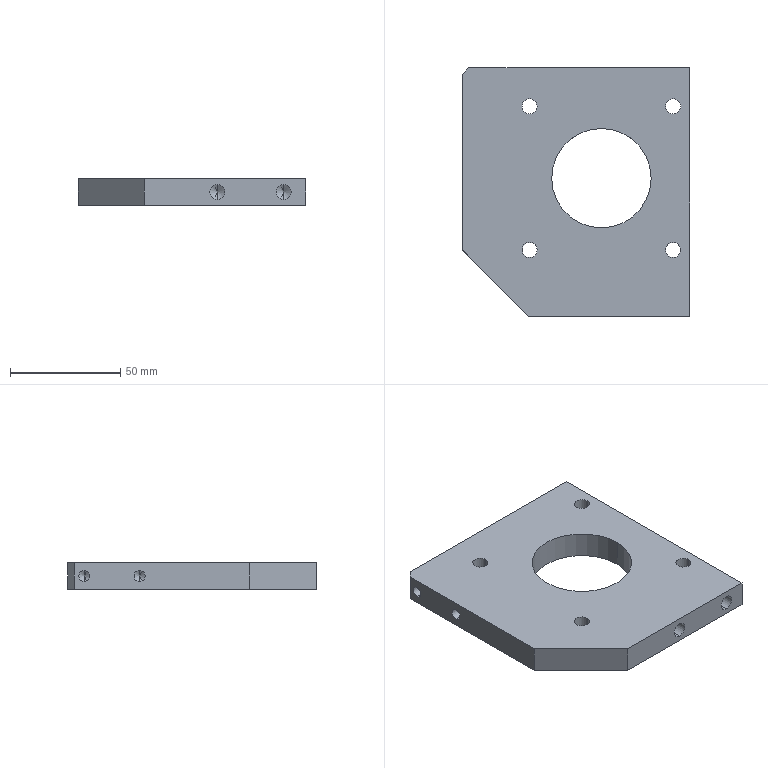Part | SolidWorks | features HoleWzd 3, Chamfer 2, ICE 2, 3DProfileFeature 1, Extrusion 1 | 1 solid | 34 faces | box 103 x 112.5 x 12 mm | volume 110488 mm3 | cylinder 18 | cone 8 | plane 8 | commonest cylinder face diameters 6.8 x12 5 x4 45 x2
STEP:
#1=CARTESIAN_POINT('',(-43.25,17.5,3.5));
#2=VERTEX_POINT('',#1);
#3=CARTESIAN_POINT('',(-43.25,17.5,8.5));
#4=VERTEX_POINT('',#3);
#5=CARTESIAN_POINT('',(-43.25,17.5,6.));
#6=DIRECTION('',(-1.,0.,0.));
#7=DIRECTION('',(0.,0.,1.));
#8=AXIS2_PLACEMENT_3D('',#5,#6,#7);
#9=CIRCLE('',#8,2.5);
#10=EDGE_CURVE('',#2,#4,#9,.T.);
#11=ORIENTED_EDGE('',*,*,#10,.F.);
#12=CARTESIAN_POINT('',(-63.,17.5,3.5));
#13=VERTEX_POINT('',#12);
#14=CARTESIAN_POINT('',(-63.,17.5,3.5));
#15=DIRECTION('',(-1.,0.,0.));
#16=VECTOR('',#15,1000.);
#17=LINE('',#14,#16);
#18=EDGE_CURVE('',#2,#13,#17,.T.);
#19=ORIENTED_EDGE('',*,*,#18,.T.);
#20=CARTESIAN_POINT('',(-63.,17.5,8.5));
#21=VERTEX_POINT('',#20);
#22=CARTESIAN_POINT('',(-63.,17.5,6.));
#23=DIRECTION('',(-1.,0.,0.));
#24=DIRECTION('',(0.,0.,1.));
#25=AXIS2_PLACEMENT_3D('',#22,#23,#24);
#26=CIRCLE('',#25,2.5);
#27=EDGE_CURVE('',#13,#21,#26,.T.);
#28=ORIENTED_EDGE('',*,*,#27,.T.);
#29=CARTESIAN_POINT('',(-63.,17.5,8.5));
#30=DIRECTION('',(-1.,0.,0.));
#31=VECTOR('',#30,1000.);
#32=LINE('',#29,#31);
#33=EDGE_CURVE('',#4,#21,#32,.T.);
#34=ORIENTED_EDGE('',*,*,#33,.F.);
#35=EDGE_LOOP('',(#11,#19,#28,#34));
#36=FACE_OUTER_BOUND('',#35,.T.);
#37=CARTESIAN_POINT('',(-63.,17.5,6.));
#38=DIRECTION('',(-1.,0.,0.));
#39=DIRECTION('',(0.,0.,1.));
#40=AXIS2_PLACEMENT_3D('',#37,#38,#39);
#41=CYLINDRICAL_SURFACE('',#40,2.5);
#42=ADVANCED_FACE('',(#36),#41,.F.);
#43=CARTESIAN_POINT('',(-41.748,17.5,6.));
#44=VERTEX_POINT('',#43);
#45=CARTESIAN_POINT('',(-43.25,17.5,8.5));
#46=DIRECTION('',(-0.515,0.,0.8572));
#47=VECTOR('',#46,1000.);
#48=LINE('',#45,#47);
#49=EDGE_CURVE('',#44,#4,#48,.T.);
#50=ORIENTED_EDGE('',*,*,#49,.F.);
#51=CARTESIAN_POINT('',(-43.25,17.5,3.5));
#52=DIRECTION('',(-0.515,0.,-0.8572));
#53=VECTOR('',#52,1000.);
#54=LINE('',#51,#53);
#55=EDGE_CURVE('',#44,#2,#54,.T.);
#56=ORIENTED_EDGE('',*,*,#55,.T.);
#57=ORIENTED_EDGE('',*,*,#10,.T.);
#58=EDGE_LOOP('',(#50,#56,#57));
#59=FACE_OUTER_BOUND('',#58,.T.);
#60=CARTESIAN_POINT('',(-43.25,17.5,6.));
#61=DIRECTION('',(-1.,0.,0.));
#62=DIRECTION('',(0.,0.,1.));
#63=AXIS2_PLACEMENT_3D('',#60,#61,#62);
#64=CONICAL_SURFACE('',#63,2.5,1.03);
#65=ADVANCED_FACE('',(#59),#64,.F.);
#66=CARTESIAN_POINT('',(-43.25,42.5,3.5));
#67=VERTEX_POINT('',#66);
#68=CARTESIAN_POINT('',(-43.25,42.5,8.5));
#69=VERTEX_POINT('',#68);
#70=CARTESIAN_POINT('',(-43.25,42.5,6.));
#71=DIRECTION('',(-1.,0.,0.));
#72=DIRECTION('',(0.,0.,1.));
#73=AXIS2_PLACEMENT_3D('',#70,#71,#72);
#74=CIRCLE('',#73,2.5);
#75=EDGE_CURVE('',#67,#69,#74,.T.);
#76=ORIENTED_EDGE('',*,*,#75,.F.);
#77=CARTESIAN_POINT('',(-63.,42.5,3.5));
#78=VERTEX_POINT('',#77);
#79=CARTESIAN_POINT('',(-63.,42.5,3.5));
#80=DIRECTION('',(-1.,0.,0.));
#81=VECTOR('',#80,1000.);
#82=LINE('',#79,#81);
#83=EDGE_CURVE('',#67,#78,#82,.T.);
#84=ORIENTED_EDGE('',*,*,#83,.T.);
#85=CARTESIAN_POINT('',(-63.,42.5,8.5));
#86=VERTEX_POINT('',#85);
#87=CARTESIAN_POINT('',(-63.,42.5,6.));
#88=DIRECTION('',(-1.,0.,0.));
#89=DIRECTION('',(0.,0.,1.));
#90=AXIS2_PLACEMENT_3D('',#87,#88,#89);
#91=CIRCLE('',#90,2.5);
#92=EDGE_CURVE('',#78,#86,#91,.T.);
#93=ORIENTED_EDGE('',*,*,#92,.T.);
#94=CARTESIAN_POINT('',(-63.,42.5,8.5));
#95=DIRECTION('',(-1.,0.,0.));
#96=VECTOR('',#95,1000.);
#97=LINE('',#94,#96);
#98=EDGE_CURVE('',#69,#86,#97,.T.);
#99=ORIENTED_EDGE('',*,*,#98,.F.);
#100=EDGE_LOOP('',(#76,#84,#93,#99));
#101=FACE_OUTER_BOUND('',#100,.T.);
#102=CARTESIAN_POINT('',(-63.,42.5,6.));
#103=DIRECTION('',(-1.,0.,0.));
#104=DIRECTION('',(0.,0.,1.));
#105=AXIS2_PLACEMENT_3D('',#102,#103,#104);
#106=CYLINDRICAL_SURFACE('',#105,2.5);
#107=ADVANCED_FACE('',(#101),#106,.F.);
#108=CARTESIAN_POINT('',(-41.748,42.5,6.));
#109=VERTEX_POINT('',#108);
#110=CARTESIAN_POINT('',(-43.25,42.5,8.5));
#111=DIRECTION('',(-0.515,0.,0.8572));
#112=VECTOR('',#111,1000.);
#113=LINE('',#110,#112);
#114=EDGE_CURVE('',#109,#69,#113,.T.);
#115=ORIENTED_EDGE('',*,*,#114,.F.);
#116=CARTESIAN_POINT('',(-43.25,42.5,3.5));
#117=DIRECTION('',(-0.515,0.,-0.8572));
#118=VECTOR('',#117,1000.);
#119=LINE('',#116,#118);
#120=EDGE_CURVE('',#109,#67,#119,.T.);
#121=ORIENTED_EDGE('',*,*,#120,.T.);
#122=ORIENTED_EDGE('',*,*,#75,.T.);
#123=EDGE_LOOP('',(#115,#121,#122));
#124=FACE_OUTER_BOUND('',#123,.T.);
#125=CARTESIAN_POINT('',(-43.25,42.5,6.));
#126=DIRECTION('',(-1.,0.,0.));
#127=DIRECTION('',(0.,0.,1.));
#128=AXIS2_PLACEMENT_3D('',#125,#126,#127);
#129=CONICAL_SURFACE('',#128,2.5,1.03);
#130=ADVANCED_FACE('',(#124),#129,.F.);
#131=CARTESIAN_POINT('',(35.9,32.5,12.));
#132=VERTEX_POINT('',#131);
#133=CARTESIAN_POINT('',(29.1,32.5,12.));
#134=VERTEX_POINT('',#133);
#135=CARTESIAN_POINT('',(32.5,32.5,12.));
#136=DIRECTION('',(0.,0.,-1.));
#137=DIRECTION('',(-1.,0.,0.));
#138=AXIS2_PLACEMENT_3D('',#135,#136,#137);
#139=CIRCLE('',#138,3.4);
#140=EDGE_CURVE('',#132,#134,#139,.T.);
#141=ORIENTED_EDGE('',*,*,#140,.F.);
#142=CARTESIAN_POINT('',(35.9,32.5,0.));
#143=VERTEX_POINT('',#142);
#144=CARTESIAN_POINT('',(35.9,32.5,0.));
#145=DIRECTION('',(0.,0.,-1.));
#146=VECTOR('',#145,1000.);
#147=LINE('',#144,#146);
#148=EDGE_CURVE('',#132,#143,#147,.T.);
#149=ORIENTED_EDGE('',*,*,#148,.T.);
#150=CARTESIAN_POINT('',(29.1,32.5,0.));
#151=VERTEX_POINT('',#150);
#152=CARTESIAN_POINT('',(32.5,32.5,0.));
#153=DIRECTION('',(0.,0.,-1.));
#154=DIRECTION('',(-1.,0.,0.));
#155=AXIS2_PLACEMENT_3D('',#152,#153,#154);
#156=CIRCLE('',#155,3.4);
#157=EDGE_CURVE('',#143,#151,#156,.T.);
#158=ORIENTED_EDGE('',*,*,#157,.T.);
#159=CARTESIAN_POINT('',(29.1,32.5,0.));
#160=DIRECTION('',(0.,0.,-1.));
#161=VECTOR('',#160,1000.);
#162=LINE('',#159,#161);
#163=EDGE_CURVE('',#134,#151,#162,.T.);
#164=ORIENTED_EDGE('',*,*,#163,.F.);
#165=EDGE_LOOP('',(#141,#149,#158,#164));
#166=FACE_OUTER_BOUND('',#165,.T.);
#167=CARTESIAN_POINT('',(32.5,32.5,0.));
#168=DIRECTION('',(0.,0.,-1.));
#169=DIRECTION('',(-1.,0.,0.));
#170=AXIS2_PLACEMENT_3D('',#167,#168,#169);
#171=CYLINDRICAL_SURFACE('',#170,3.4);
#172=ADVANCED_FACE('',(#166),#171,.F.);
#173=CARTESIAN_POINT('',(-29.1,32.5,12.));
#174=VERTEX_POINT('',#173);
#175=CARTESIAN_POINT('',(-35.9,32.5,12.));
#176=VERTEX_POINT('',#175);
#177=CARTESIAN_POINT('',(-32.5,32.5,12.));
#178=DIRECTION('',(0.,0.,-1.));
#179=DIRECTION('',(-1.,0.,0.));
#180=AXIS2_PLACEMENT_3D('',#177,#178,#179);
#181=CIRCLE('',#180,3.4);
#182=EDGE_CURVE('',#174,#176,#181,.T.);
#183=ORIENTED_EDGE('',*,*,#182,.F.);
#184=CARTESIAN_POINT('',(-29.1,32.5,0.));
#185=VERTEX_POINT('',#184);
#186=CARTESIAN_POINT('',(-29.1,32.5,0.));
#187=DIRECTION('',(0.,0.,-1.));
#188=VECTOR('',#187,1000.);
#189=LINE('',#186,#188);
#190=EDGE_CURVE('',#174,#185,#189,.T.);
#191=ORIENTED_EDGE('',*,*,#190,.T.);
#192=CARTESIAN_POINT('',(-35.9,32.5,0.));
#193=VERTEX_POINT('',#192);
#194=CARTESIAN_POINT('',(-32.5,32.5,0.));
#195=DIRECTION('',(0.,0.,-1.));
#196=DIRECTION('',(-1.,0.,0.));
#197=AXIS2_PLACEMENT_3D('',#194,#195,#196);
#198=CIRCLE('',#197,3.4);
#199=EDGE_CURVE('',#185,#193,#198,.T.);
#200=ORIENTED_EDGE('',*,*,#199,.T.);
#201=CARTESIAN_POINT('',(-35.9,32.5,0.));
#202=DIRECTION('',(0.,0.,-1.));
#203=VECTOR('',#202,1000.);
#204=LINE('',#201,#203);
#205=EDGE_CURVE('',#176,#193,#204,.T.);
#206=ORIENTED_EDGE('',*,*,#205,.F.);
#207=EDGE_LOOP('',(#183,#191,#200,#206));
#208=FACE_OUTER_BOUND('',#207,.T.);
#209=CARTESIAN_POINT('',(-32.5,32.5,0.));
#210=DIRECTION('',(0.,0.,-1.));
#211=DIRECTION('',(-1.,0.,0.));
#212=AXIS2_PLACEMENT_3D('',#209,#210,#211);
#213=CYLINDRICAL_SURFACE('',#212,3.4);
#214=ADVANCED_FACE('',(#208),#213,.F.);
#215=CARTESIAN_POINT('',(-29.1,-32.5,12.));
#216=VERTEX_POINT('',#215);
#217=CARTESIAN_POINT('',(-35.9,-32.5,12.));
#218=VERTEX_POINT('',#217);
#219=CARTESIAN_POINT('',(-32.5,-32.5,12.));
#220=DIRECTION('',(0.,0.,-1.));
#221=DIRECTION('',(-1.,0.,0.));
#222=AXIS2_PLACEMENT_3D('',#219,#220,#221);
#223=CIRCLE('',#222,3.4);
#224=EDGE_CURVE('',#216,#218,#223,.T.);
#225=ORIENTED_EDGE('',*,*,#224,.F.);
#226=CARTESIAN_POINT('',(-29.1,-32.5,0.));
#227=VERTEX_POINT('',#226);
#228=CARTESIAN_POINT('',(-29.1,-32.5,0.));
#229=DIRECTION('',(0.,0.,-1.));
#230=VECTOR('',#229,1000.);
#231=LINE('',#228,#230);
#232=EDGE_CURVE('',#216,#227,#231,.T.);
#233=ORIENTED_EDGE('',*,*,#232,.T.);
#234=CARTESIAN_POINT('',(-35.9,-32.5,0.));
#235=VERTEX_POINT('',#234);
#236=CARTESIAN_POINT('',(-32.5,-32.5,0.));
#237=DIRECTION('',(0.,0.,-1.));
#238=DIRECTION('',(-1.,0.,0.));
#239=AXIS2_PLACEMENT_3D('',#236,#237,#238);
#240=CIRCLE('',#239,3.4);
#241=EDGE_CURVE('',#227,#235,#240,.T.);
#242=ORIENTED_EDGE('',*,*,#241,.T.);
#243=CARTESIAN_POINT('',(-35.9,-32.5,0.));
#244=DIRECTION('',(0.,0.,-1.));
#245=VECTOR('',#244,1000.);
#246=LINE('',#243,#245);
#247=EDGE_CURVE('',#218,#235,#246,.T.);
#248=ORIENTED_EDGE('',*,*,#247,.F.);
#249=EDGE_LOOP('',(#225,#233,#242,#248));
#250=FACE_OUTER_BOUND('',#249,.T.);
#251=CARTESIAN_POINT('',(-32.5,-32.5,0.));
#252=DIRECTION('',(0.,0.,-1.));
#253=DIRECTION('',(-1.,0.,0.));
#254=AXIS2_PLACEMENT_3D('',#251,#252,#253);
#255=CYLINDRICAL_SURFACE('',#254,3.4);
#256=ADVANCED_FACE('',(#250),#255,.F.);
#257=CARTESIAN_POINT('',(35.9,-32.5,12.));
#258=VERTEX_POINT('',#257);
#259=CARTESIAN_POINT('',(29.1,-32.5,12.));
#260=VERTEX_POINT('',#259);
#261=CARTESIAN_POINT('',(32.5,-32.5,12.));
#262=DIRECTION('',(0.,0.,-1.));
#263=DIRECTION('',(-1.,0.,0.));
#264=AXIS2_PLACEMENT_3D('',#261,#262,#263);
#265=CIRCLE('',#264,3.4);
#266=EDGE_CURVE('',#258,#260,#265,.T.);
#267=ORIENTED_EDGE('',*,*,#266,.F.);
#268=CARTESIAN_POINT('',(35.9,-32.5,0.));
#269=VERTEX_POINT('',#268);
#270=CARTESIAN_POINT('',(35.9,-32.5,0.));
#271=DIRECTION('',(0.,0.,-1.));
#272=VECTOR('',#271,1000.);
#273=LINE('',#270,#272);
#274=EDGE_CURVE('',#258,#269,#273,.T.);
#275=ORIENTED_EDGE('',*,*,#274,.T.);
#276=CARTESIAN_POINT('',(29.1,-32.5,0.));
#277=VERTEX_POINT('',#276);
#278=CARTESIAN_POINT('',(32.5,-32.5,0.));
#279=DIRECTION('',(0.,0.,-1.));
#280=DIRECTION('',(-1.,0.,0.));
#281=AXIS2_PLACEMENT_3D('',#278,#279,#280);
#282=CIRCLE('',#281,3.4);
#283=EDGE_CURVE('',#269,#277,#282,.T.);
#284=ORIENTED_EDGE('',*,*,#283,.T.);
#285=CARTESIAN_POINT('',(29.1,-32.5,0.));
#286=DIRECTION('',(0.,0.,-1.));
#287=VECTOR('',#286,1000.);
#288=LINE('',#285,#287);
#289=EDGE_CURVE('',#260,#277,#288,.T.);
#290=ORIENTED_EDGE('',*,*,#289,.F.);
#291=EDGE_LOOP('',(#267,#275,#284,#290));
#292=FACE_OUTER_BOUND('',#291,.T.);
#293=CARTESIAN_POINT('',(32.5,-32.5,0.));
#294=DIRECTION('',(0.,0.,-1.));
#295=DIRECTION('',(-1.,0.,0.));
#296=AXIS2_PLACEMENT_3D('',#293,#294,#295);
#297=CYLINDRICAL_SURFACE('',#296,3.4);
#298=ADVANCED_FACE('',(#292),#297,.F.);
#299=CARTESIAN_POINT('',(30.,-42.75,9.4));
#300=VERTEX_POINT('',#299);
#301=CARTESIAN_POINT('',(30.,-42.75,2.6));
#302=VERTEX_POINT('',#301);
#303=CARTESIAN_POINT('',(30.,-42.75,6.));
#304=DIRECTION('',(0.,-1.,0.));
#305=DIRECTION('',(0.,0.,-1.));
#306=AXIS2_PLACEMENT_3D('',#303,#304,#305);
#307=CIRCLE('',#306,3.4);
#308=EDGE_CURVE('',#300,#302,#307,.T.);
#309=ORIENTED_EDGE('',*,*,#308,.F.);
#310=CARTESIAN_POINT('',(30.,-62.5,9.4));
#311=VERTEX_POINT('',#310);
#312=CARTESIAN_POINT('',(30.,-62.5,9.4));
#313=DIRECTION('',(0.,-1.,0.));
#314=VECTOR('',#313,1000.);
#315=LINE('',#312,#314);
#316=EDGE_CURVE('',#300,#311,#315,.T.);
#317=ORIENTED_EDGE('',*,*,#316,.T.);
#318=CARTESIAN_POINT('',(30.,-62.5,2.6));
#319=VERTEX_POINT('',#318);
#320=CARTESIAN_POINT('',(30.,-62.5,6.));
#321=DIRECTION('',(0.,-1.,0.));
#322=DIRECTION('',(0.,0.,-1.));
#323=AXIS2_PLACEMENT_3D('',#320,#321,#322);
#324=CIRCLE('',#323,3.4);
#325=EDGE_CURVE('',#311,#319,#324,.T.);
#326=ORIENTED_EDGE('',*,*,#325,.T.);
#327=CARTESIAN_POINT('',(30.,-62.5,2.6));
#328=DIRECTION('',(0.,-1.,0.));
#329=VECTOR('',#328,1000.);
#330=LINE('',#327,#329);
#331=EDGE_CURVE('',#302,#319,#330,.T.);
#332=ORIENTED_EDGE('',*,*,#331,.F.);
#333=EDGE_LOOP('',(#309,#317,#326,#332));
#334=FACE_OUTER_BOUND('',#333,.T.);
#335=CARTESIAN_POINT('',(30.,-62.5,6.));
#336=DIRECTION('',(0.,-1.,0.));
#337=DIRECTION('',(0.,0.,-1.));
#338=AXIS2_PLACEMENT_3D('',#335,#336,#337);
#339=CYLINDRICAL_SURFACE('',#338,3.4);
#340=ADVANCED_FACE('',(#334),#339,.F.);
#341=CARTESIAN_POINT('',(30.,-40.707,6.));
#342=VERTEX_POINT('',#341);
#343=CARTESIAN_POINT('',(30.,-42.75,2.6));
#344=DIRECTION('',(0.,-0.515,-0.8572));
#345=VECTOR('',#344,1000.);
#346=LINE('',#343,#345);
#347=EDGE_CURVE('',#342,#302,#346,.T.);
#348=ORIENTED_EDGE('',*,*,#347,.F.);
#349=CARTESIAN_POINT('',(30.,-42.75,9.4));
#350=DIRECTION('',(0.,-0.515,0.8572));
#351=VECTOR('',#350,1000.);
#352=LINE('',#349,#351);
#353=EDGE_CURVE('',#342,#300,#352,.T.);
#354=ORIENTED_EDGE('',*,*,#353,.T.);
#355=ORIENTED_EDGE('',*,*,#308,.T.);
#356=EDGE_LOOP('',(#348,#354,#355));
#357=FACE_OUTER_BOUND('',#356,.T.);
#358=CARTESIAN_POINT('',(30.,-42.75,6.));
#359=DIRECTION('',(0.,-1.,0.));
#360=DIRECTION('',(0.,0.,-1.));
#361=AXIS2_PLACEMENT_3D('',#358,#359,#360);
#362=CONICAL_SURFACE('',#361,3.4,1.03);
#363=ADVANCED_FACE('',(#357),#362,.F.);
#364=CARTESIAN_POINT('',(0.,-42.75,9.4));
#365=VERTEX_POINT('',#364);
#366=CARTESIAN_POINT('',(0.,-42.75,2.6));
#367=VERTEX_POINT('',#366);
#368=CARTESIAN_POINT('',(0.,-42.75,6.));
#369=DIRECTION('',(0.,-1.,0.));
#370=DIRECTION('',(0.,0.,-1.));
#371=AXIS2_PLACEMENT_3D('',#368,#369,#370);
#372=CIRCLE('',#371,3.4);
#373=EDGE_CURVE('',#365,#367,#372,.T.);
#374=ORIENTED_EDGE('',*,*,#373,.F.);
#375=CARTESIAN_POINT('',(0.,-62.5,9.4));
#376=VERTEX_POINT('',#375);
#377=CARTESIAN_POINT('',(0.,-62.5,9.4));
#378=DIRECTION('',(0.,-1.,0.));
#379=VECTOR('',#378,1000.);
#380=LINE('',#377,#379);
#381=EDGE_CURVE('',#365,#376,#380,.T.);
#382=ORIENTED_EDGE('',*,*,#381,.T.);
#383=CARTESIAN_POINT('',(0.,-62.5,2.6));
#384=VERTEX_POINT('',#383);
#385=CARTESIAN_POINT('',(0.,-62.5,6.));
#386=DIRECTION('',(0.,-1.,0.));
#387=DIRECTION('',(0.,0.,-1.));
#388=AXIS2_PLACEMENT_3D('',#385,#386,#387);
#389=CIRCLE('',#388,3.4);
#390=EDGE_CURVE('',#376,#384,#389,.T.);
#391=ORIENTED_EDGE('',*,*,#390,.T.);
#392=CARTESIAN_POINT('',(0.,-62.5,2.6));
#393=DIRECTION('',(0.,-1.,0.));
#394=VECTOR('',#393,1000.);
#395=LINE('',#392,#394);
#396=EDGE_CURVE('',#367,#384,#395,.T.);
#397=ORIENTED_EDGE('',*,*,#396,.F.);
#398=EDGE_LOOP('',(#374,#382,#391,#397));
#399=FACE_OUTER_BOUND('',#398,.T.);
#400=CARTESIAN_POINT('',(0.,-62.5,6.));
#401=DIRECTION('',(0.,-1.,0.));
#402=DIRECTION('',(0.,0.,-1.));
#403=AXIS2_PLACEMENT_3D('',#400,#401,#402);
#404=CYLINDRICAL_SURFACE('',#403,3.4);
#405=ADVANCED_FACE('',(#399),#404,.F.);
#406=CARTESIAN_POINT('',(0.,-40.707,6.));
#407=VERTEX_POINT('',#406);
#408=CARTESIAN_POINT('',(0.,-42.75,2.6));
#409=DIRECTION('',(0.,-0.515,-0.8572));
#410=VECTOR('',#409,1000.);
#411=LINE('',#408,#410);
#412=EDGE_CURVE('',#407,#367,#411,.T.);
#413=ORIENTED_EDGE('',*,*,#412,.F.);
#414=CARTESIAN_POINT('',(0.,-42.75,9.4));
#415=DIRECTION('',(0.,-0.515,0.8572));
#416=VECTOR('',#415,1000.);
#417=LINE('',#414,#416);
#418=EDGE_CURVE('',#407,#365,#417,.T.);
#419=ORIENTED_EDGE('',*,*,#418,.T.);
#420=ORIENTED_EDGE('',*,*,#373,.T.);
#421=EDGE_LOOP('',(#413,#419,#420));
#422=FACE_OUTER_BOUND('',#421,.T.);
#423=CARTESIAN_POINT('',(0.,-42.75,6.));
#424=DIRECTION('',(0.,-1.,0.));
#425=DIRECTION('',(0.,0.,-1.));
#426=AXIS2_PLACEMENT_3D('',#423,#424,#425);
#427=CONICAL_SURFACE('',#426,3.4,1.03);
#428=ADVANCED_FACE('',(#422),#427,.F.);
#429=CARTESIAN_POINT('',(-22.5,0.,12.));
#430=VERTEX_POINT('',#429);
#431=CARTESIAN_POINT('',(22.5,0.,12.));
#432=VERTEX_POINT('',#431);
#433=CARTESIAN_POINT('',(0.,0.,12.));
#434=DIRECTION('',(0.,0.,1.));
#435=DIRECTION('',(1.,0.,0.));
#436=AXIS2_PLACEMENT_3D('',#433,#434,#435);
#437=CIRCLE('',#436,22.5);
#438=EDGE_CURVE('',#430,#432,#437,.T.);
#439=ORIENTED_EDGE('',*,*,#438,.T.);
#440=CARTESIAN_POINT('',(22.5,0.,0.));
#441=VERTEX_POINT('',#440);
#442=CARTESIAN_POINT('',(22.5,0.,12.));
#443=DIRECTION('',(0.,0.,-1.));
#444=VECTOR('',#443,1000.);
#445=LINE('',#442,#444);
#446=EDGE_CURVE('',#432,#441,#445,.T.);
#447=ORIENTED_EDGE('',*,*,#446,.T.);
#448=CARTESIAN_POINT('',(-22.5,0.,0.));
#449=VERTEX_POINT('',#448);
#450=CARTESIAN_POINT('',(0.,0.,0.));
#451=DIRECTION('',(0.,0.,1.));
#452=DIRECTION('',(1.,0.,0.));
#453=AXIS2_PLACEMENT_3D('',#450,#451,#452);
#454=CIRCLE('',#453,22.5);
#455=EDGE_CURVE('',#449,#441,#454,.T.);
#456=ORIENTED_EDGE('',*,*,#455,.F.);
#457=CARTESIAN_POINT('',(-22.5,0.,12.));
#458=DIRECTION('',(0.,0.,-1.));
#459=VECTOR('',#458,1000.);
#460=LINE('',#457,#459);
#461=EDGE_CURVE('',#430,#449,#460,.T.);
#462=ORIENTED_EDGE('',*,*,#461,.F.);
#463=EDGE_LOOP('',(#439,#447,#456,#462));
#464=FACE_OUTER_BOUND('',#463,.T.);
#465=CARTESIAN_POINT('',(0.,0.,12.));
#466=DIRECTION('',(0.,0.,-1.));
#467=DIRECTION('',(-1.,0.,0.));
#468=AXIS2_PLACEMENT_3D('',#465,#466,#467);
#469=CYLINDRICAL_SURFACE('',#468,22.5);
#470=ADVANCED_FACE('',(#464),#469,.F.);
#471=CARTESIAN_POINT('',(32.5,32.5,12.));
#472=DIRECTION('',(0.,0.,-1.));
#473=DIRECTION('',(-1.,0.,0.));
#474=AXIS2_PLACEMENT_3D('',#471,#472,#473);
#475=CIRCLE('',#474,3.4);
#476=EDGE_CURVE('',#134,#132,#475,.T.);
#477=ORIENTED_EDGE('',*,*,#476,.T.);
#478=ORIENTED_EDGE('',*,*,#140,.T.);
#479=EDGE_LOOP('',(#477,#478));
#480=FACE_BOUND('',#479,.T.);
#481=CARTESIAN_POINT('',(-32.5,32.5,12.));
#482=DIRECTION('',(0.,0.,-1.));
#483=DIRECTION('',(-1.,0.,0.));
#484=AXIS2_PLACEMENT_3D('',#481,#482,#483);
#485=CIRCLE('',#484,3.4);
#486=EDGE_CURVE('',#176,#174,#485,.T.);
#487=ORIENTED_EDGE('',*,*,#486,.T.);
#488=ORIENTED_EDGE('',*,*,#182,.T.);
#489=EDGE_LOOP('',(#487,#488));
#490=FACE_BOUND('',#489,.T.);
#491=CARTESIAN_POINT('',(-32.5,-32.5,12.));
#492=DIRECTION('',(0.,0.,-1.));
#493=DIRECTION('',(-1.,0.,0.));
#494=AXIS2_PLACEMENT_3D('',#491,#492,#493);
#495=CIRCLE('',#494,3.4);
#496=EDGE_CURVE('',#218,#216,#495,.T.);
#497=ORIENTED_EDGE('',*,*,#496,.T.);
#498=ORIENTED_EDGE('',*,*,#224,.T.);
#499=EDGE_LOOP('',(#497,#498));
#500=FACE_BOUND('',#499,.T.);
#501=CARTESIAN_POINT('',(32.5,-32.5,12.));
#502=DIRECTION('',(0.,0.,-1.));
#503=DIRECTION('',(-1.,0.,0.));
#504=AXIS2_PLACEMENT_3D('',#501,#502,#503);
#505=CIRCLE('',#504,3.4);
#506=EDGE_CURVE('',#260,#258,#505,.T.);
#507=ORIENTED_EDGE('',*,*,#506,.T.);
#508=ORIENTED_EDGE('',*,*,#266,.T.);
#509=EDGE_LOOP('',(#507,#508));
#510=FACE_BOUND('',#509,.T.);
#511=CARTESIAN_POINT('',(-33.,-62.5,12.));
#512=VERTEX_POINT('',#511);
#513=CARTESIAN_POINT('',(40.,-62.5,12.));
#514=VERTEX_POINT('',#513);
#515=CARTESIAN_POINT('',(45.,-62.5,12.));
#516=DIRECTION('',(1.,0.,0.));
#517=VECTOR('',#516,1000.);
#518=LINE('',#515,#517);
#519=EDGE_CURVE('',#512,#514,#518,.T.);
#520=ORIENTED_EDGE('',*,*,#519,.T.);
#521=CARTESIAN_POINT('',(40.,50.,12.));
#522=VERTEX_POINT('',#521);
#523=CARTESIAN_POINT('',(40.,0.,12.));
#524=DIRECTION('',(0.,1.,0.));
#525=VECTOR('',#524,1000.);
#526=LINE('',#523,#525);
#527=EDGE_CURVE('',#514,#522,#526,.T.);
#528=ORIENTED_EDGE('',*,*,#527,.T.);
#529=CARTESIAN_POINT('',(-60.,50.,12.));
#530=VERTEX_POINT('',#529);
#531=CARTESIAN_POINT('',(-63.,50.,12.));
#532=DIRECTION('',(1.,0.,0.));
#533=VECTOR('',#532,1000.);
#534=LINE('',#531,#533);
#535=EDGE_CURVE('',#530,#522,#534,.T.);
#536=ORIENTED_EDGE('',*,*,#535,.F.);
#537=CARTESIAN_POINT('',(-63.,47.,12.));
#538=VERTEX_POINT('',#537);
#539=CARTESIAN_POINT('',(-60.,50.,12.));
#540=DIRECTION('',(-0.7071,-0.7071,0.));
#541=VECTOR('',#540,1000.);
#542=LINE('',#539,#541);
#543=EDGE_CURVE('',#530,#538,#542,.T.);
#544=ORIENTED_EDGE('',*,*,#543,.T.);
#545=CARTESIAN_POINT('',(-63.,-32.5,12.));
#546=VERTEX_POINT('',#545);
#547=CARTESIAN_POINT('',(-63.,47.5,12.));
#548=DIRECTION('',(0.,-1.,0.));
#549=VECTOR('',#548,1000.);
#550=LINE('',#547,#549);
#551=EDGE_CURVE('',#538,#546,#550,.T.);
#552=ORIENTED_EDGE('',*,*,#551,.T.);
#553=CARTESIAN_POINT('',(-33.,-62.5,12.));
#554=DIRECTION('',(0.7071,-0.7071,0.));
#555=VECTOR('',#554,1000.);
#556=LINE('',#553,#555);
#557=EDGE_CURVE('',#546,#512,#556,.T.);
#558=ORIENTED_EDGE('',*,*,#557,.T.);
#559=EDGE_LOOP('',(#520,#528,#536,#544,#552,#558));
#560=FACE_OUTER_BOUND('',#559,.T.);
#561=ORIENTED_EDGE('',*,*,#438,.F.);
#562=CARTESIAN_POINT('',(0.,0.,12.));
#563=DIRECTION('',(0.,0.,1.));
#564=DIRECTION('',(1.,0.,0.));
#565=AXIS2_PLACEMENT_3D('',#562,#563,#564);
#566=CIRCLE('',#565,22.5);
#567=EDGE_CURVE('',#432,#430,#566,.T.);
#568=ORIENTED_EDGE('',*,*,#567,.F.);
#569=EDGE_LOOP('',(#561,#568));
#570=FACE_BOUND('',#569,.T.);
#571=CARTESIAN_POINT('',(0.,0.,12.));
#572=DIRECTION('',(0.,0.,-1.));
#573=DIRECTION('',(-1.,0.,0.));
#574=AXIS2_PLACEMENT_3D('',#571,#572,#573);
#575=PLANE('',#574);
#576=ADVANCED_FACE('',(#480,#490,#500,#510,#560,#570),#575,.F.);
#577=CARTESIAN_POINT('',(40.,-62.5,0.));
#578=VERTEX_POINT('',#577);
#579=CARTESIAN_POINT('',(40.,50.,0.));
#580=VERTEX_POINT('',#579);
#581=CARTESIAN_POINT('',(40.,50.,0.));
#582=DIRECTION('',(0.,1.,0.));
#583=VECTOR('',#582,1000.);
#584=LINE('',#581,#583);
#585=EDGE_CURVE('',#578,#580,#584,.T.);
#586=ORIENTED_EDGE('',*,*,#585,.F.);
#587=CARTESIAN_POINT('',(-33.,-62.5,0.));
#588=VERTEX_POINT('',#587);
#589=CARTESIAN_POINT('',(45.,-62.5,0.));
#590=DIRECTION('',(1.,0.,0.));
#591=VECTOR('',#590,1000.);
#592=LINE('',#589,#591);
#593=EDGE_CURVE('',#588,#578,#592,.T.);
#594=ORIENTED_EDGE('',*,*,#593,.F.);
#595=CARTESIAN_POINT('',(-63.,-32.5,0.));
#596=VERTEX_POINT('',#595);
#597=CARTESIAN_POINT('',(-47.75,-47.75,0.));
#598=DIRECTION('',(-0.7071,0.7071,0.));
#599=VECTOR('',#598,1000.);
#600=LINE('',#597,#599);
#601=EDGE_CURVE('',#588,#596,#600,.T.);
#602=ORIENTED_EDGE('',*,*,#601,.T.);
#603=CARTESIAN_POINT('',(-63.,47.,0.));
#604=VERTEX_POINT('',#603);
#605=CARTESIAN_POINT('',(-63.,-62.5,0.));
#606=DIRECTION('',(0.,-1.,0.));
#607=VECTOR('',#606,1000.);
#608=LINE('',#605,#607);
#609=EDGE_CURVE('',#604,#596,#608,.T.);
#610=ORIENTED_EDGE('',*,*,#609,.F.);
#611=CARTESIAN_POINT('',(-60.,50.,0.));
#612=VERTEX_POINT('',#611);
#613=CARTESIAN_POINT('',(-55.,55.,0.));
#614=DIRECTION('',(0.7071,0.7071,0.));
#615=VECTOR('',#614,1000.);
#616=LINE('',#613,#615);
#617=EDGE_CURVE('',#604,#612,#616,.T.);
#618=ORIENTED_EDGE('',*,*,#617,.T.);
#619=CARTESIAN_POINT('',(45.,50.,0.));
#620=DIRECTION('',(-1.,0.,0.));
#621=VECTOR('',#620,1000.);
#622=LINE('',#619,#621);
#623=EDGE_CURVE('',#580,#612,#622,.T.);
#624=ORIENTED_EDGE('',*,*,#623,.F.);
#625=EDGE_LOOP('',(#586,#594,#602,#610,#618,#624));
#626=FACE_OUTER_BOUND('',#625,.T.);
#627=CARTESIAN_POINT('',(32.5,32.5,0.));
#628=DIRECTION('',(0.,0.,-1.));
#629=DIRECTION('',(-1.,0.,0.));
#630=AXIS2_PLACEMENT_3D('',#627,#628,#629);
#631=CIRCLE('',#630,3.4);
#632=EDGE_CURVE('',#151,#143,#631,.T.);
#633=ORIENTED_EDGE('',*,*,#632,.F.);
#634=ORIENTED_EDGE('',*,*,#157,.F.);
#635=EDGE_LOOP('',(#633,#634));
#636=FACE_BOUND('',#635,.T.);
#637=CARTESIAN_POINT('',(-32.5,32.5,0.));
#638=DIRECTION('',(0.,0.,-1.));
#639=DIRECTION('',(-1.,0.,0.));
#640=AXIS2_PLACEMENT_3D('',#637,#638,#639);
#641=CIRCLE('',#640,3.4);
#642=EDGE_CURVE('',#193,#185,#641,.T.);
#643=ORIENTED_EDGE('',*,*,#642,.F.);
#644=ORIENTED_EDGE('',*,*,#199,.F.);
#645=EDGE_LOOP('',(#643,#644));
#646=FACE_BOUND('',#645,.T.);
#647=CARTESIAN_POINT('',(-32.5,-32.5,0.));
#648=DIRECTION('',(0.,0.,-1.));
#649=DIRECTION('',(-1.,0.,0.));
#650=AXIS2_PLACEMENT_3D('',#647,#648,#649);
#651=CIRCLE('',#650,3.4);
#652=EDGE_CURVE('',#235,#227,#651,.T.);
#653=ORIENTED_EDGE('',*,*,#652,.F.);
#654=ORIENTED_EDGE('',*,*,#241,.F.);
#655=EDGE_LOOP('',(#653,#654));
#656=FACE_BOUND('',#655,.T.);
#657=CARTESIAN_POINT('',(32.5,-32.5,0.));
#658=DIRECTION('',(0.,0.,-1.));
#659=DIRECTION('',(-1.,0.,0.));
#660=AXIS2_PLACEMENT_3D('',#657,#658,#659);
#661=CIRCLE('',#660,3.4);
#662=EDGE_CURVE('',#277,#269,#661,.T.);
#663=ORIENTED_EDGE('',*,*,#662,.F.);
#664=ORIENTED_EDGE('',*,*,#283,.F.);
#665=EDGE_LOOP('',(#663,#664));
#666=FACE_BOUND('',#665,.T.);
#667=ORIENTED_EDGE('',*,*,#455,.T.);
#668=CARTESIAN_POINT('',(0.,0.,0.));
#669=DIRECTION('',(0.,0.,1.));
#670=DIRECTION('',(1.,0.,0.));
#671=AXIS2_PLACEMENT_3D('',#668,#669,#670);
#672=CIRCLE('',#671,22.5);
#673=EDGE_CURVE('',#441,#449,#672,.T.);
#674=ORIENTED_EDGE('',*,*,#673,.T.);
#675=EDGE_LOOP('',(#667,#674));
#676=FACE_BOUND('',#675,.T.);
#677=CARTESIAN_POINT('',(0.,0.,0.));
#678=DIRECTION('',(0.,0.,-1.));
#679=DIRECTION('',(-1.,0.,0.));
#680=AXIS2_PLACEMENT_3D('',#677,#678,#679);
#681=PLANE('',#680);
#682=ADVANCED_FACE('',(#626,#636,#646,#656,#666,#676),#681,.T.);
#683=CARTESIAN_POINT('',(-63.,17.5,6.));
#684=DIRECTION('',(-1.,0.,0.));
#685=DIRECTION('',(0.,0.,1.));
#686=AXIS2_PLACEMENT_3D('',#683,#684,#685);
#687=CIRCLE('',#686,2.5);
#688=EDGE_CURVE('',#21,#13,#687,.T.);
#689=ORIENTED_EDGE('',*,*,#688,.F.);
#690=ORIENTED_EDGE('',*,*,#27,.F.);
#691=EDGE_LOOP('',(#689,#690));
#692=FACE_BOUND('',#691,.T.);
#693=CARTESIAN_POINT('',(-63.,42.5,6.));
#694=DIRECTION('',(-1.,0.,0.));
#695=DIRECTION('',(0.,0.,1.));
#696=AXIS2_PLACEMENT_3D('',#693,#694,#695);
#697=CIRCLE('',#696,2.5);
#698=EDGE_CURVE('',#86,#78,#697,.T.);
#699=ORIENTED_EDGE('',*,*,#698,.F.);
#700=ORIENTED_EDGE('',*,*,#92,.F.);
#701=EDGE_LOOP('',(#699,#700));
#702=FACE_BOUND('',#701,.T.);
#703=ORIENTED_EDGE('',*,*,#551,.F.);
#704=CARTESIAN_POINT('',(-63.,47.,0.));
#705=DIRECTION('',(0.,0.,-1.));
#706=VECTOR('',#705,1000.);
#707=LINE('',#704,#706);
#708=EDGE_CURVE('',#538,#604,#707,.T.);
#709=ORIENTED_EDGE('',*,*,#708,.T.);
#710=ORIENTED_EDGE('',*,*,#609,.T.);
#711=CARTESIAN_POINT('',(-63.,-32.5,12.));
#712=DIRECTION('',(0.,0.,1.));
#713=VECTOR('',#712,1000.);
#714=LINE('',#711,#713);
#715=EDGE_CURVE('',#596,#546,#714,.T.);
#716=ORIENTED_EDGE('',*,*,#715,.T.);
#717=EDGE_LOOP('',(#703,#709,#710,#716));
#718=FACE_OUTER_BOUND('',#717,.T.);
#719=CARTESIAN_POINT('',(-63.,-62.5,12.));
#720=DIRECTION('',(1.,0.,0.));
#721=DIRECTION('',(0.,0.,-1.));
#722=AXIS2_PLACEMENT_3D('',#719,#720,#721);
#723=PLANE('',#722);
#724=ADVANCED_FACE('',(#692,#702,#718),#723,.F.);
#725=CARTESIAN_POINT('',(30.,-62.5,6.));
#726=DIRECTION('',(0.,-1.,0.));
#727=DIRECTION('',(0.,0.,-1.));
#728=AXIS2_PLACEMENT_3D('',#725,#726,#727);
#729=CIRCLE('',#728,3.4);
#730=EDGE_CURVE('',#319,#311,#729,.T.);
#731=ORIENTED_EDGE('',*,*,#730,.F.);
#732=ORIENTED_EDGE('',*,*,#325,.F.);
#733=EDGE_LOOP('',(#731,#732));
#734=FACE_BOUND('',#733,.T.);
#735=CARTESIAN_POINT('',(0.,-62.5,6.));
#736=DIRECTION('',(0.,-1.,0.));
#737=DIRECTION('',(0.,0.,-1.));
#738=AXIS2_PLACEMENT_3D('',#735,#736,#737);
#739=CIRCLE('',#738,3.4);
#740=EDGE_CURVE('',#384,#376,#739,.T.);
#741=ORIENTED_EDGE('',*,*,#740,.F.);
#742=ORIENTED_EDGE('',*,*,#390,.F.);
#743=EDGE_LOOP('',(#741,#742));
#744=FACE_BOUND('',#743,.T.);
#745=ORIENTED_EDGE('',*,*,#593,.T.);
#746=CARTESIAN_POINT('',(40.,-62.5,15.));
#747=DIRECTION('',(0.,0.,-1.));
#748=VECTOR('',#747,1000.);
#749=LINE('',#746,#748);
#750=EDGE_CURVE('',#514,#578,#749,.T.);
#751=ORIENTED_EDGE('',*,*,#750,.F.);
#752=ORIENTED_EDGE('',*,*,#519,.F.);
#753=CARTESIAN_POINT('',(-33.,-62.5,12.));
#754=DIRECTION('',(0.,0.,-1.));
#755=VECTOR('',#754,1000.);
#756=LINE('',#753,#755);
#757=EDGE_CURVE('',#512,#588,#756,.T.);
#758=ORIENTED_EDGE('',*,*,#757,.T.);
#759=EDGE_LOOP('',(#745,#751,#752,#758));
#760=FACE_OUTER_BOUND('',#759,.T.);
#761=CARTESIAN_POINT('',(45.,-62.5,12.));
#762=DIRECTION('',(0.,1.,0.));
#763=DIRECTION('',(-1.,0.,0.));
#764=AXIS2_PLACEMENT_3D('',#761,#762,#763);
#765=PLANE('',#764);
#766=ADVANCED_FACE('',(#734,#744,#760),#765,.F.);
#767=ORIENTED_EDGE('',*,*,#446,.F.);
#768=ORIENTED_EDGE('',*,*,#567,.T.);
#769=ORIENTED_EDGE('',*,*,#461,.T.);
#770=ORIENTED_EDGE('',*,*,#673,.F.);
#771=EDGE_LOOP('',(#767,#768,#769,#770));
#772=FACE_OUTER_BOUND('',#771,.T.);
#773=CARTESIAN_POINT('',(0.,0.,12.));
#774=DIRECTION('',(0.,0.,-1.));
#775=DIRECTION('',(-1.,0.,0.));
#776=AXIS2_PLACEMENT_3D('',#773,#774,#775);
#777=CYLINDRICAL_SURFACE('',#776,22.5);
#778=ADVANCED_FACE('',(#772),#777,.F.);
#779=ORIENTED_EDGE('',*,*,#557,.F.);
#780=ORIENTED_EDGE('',*,*,#715,.F.);
#781=ORIENTED_EDGE('',*,*,#601,.F.);
#782=ORIENTED_EDGE('',*,*,#757,.F.);
#783=EDGE_LOOP('',(#779,#780,#781,#782));
#784=FACE_OUTER_BOUND('',#783,.T.);
#785=CARTESIAN_POINT('',(-33.,-62.5,12.));
#786=DIRECTION('',(0.7071,0.7071,0.));
#787=DIRECTION('',(0.,0.,-1.));
#788=AXIS2_PLACEMENT_3D('',#785,#786,#787);
#789=PLANE('',#788);
#790=ADVANCED_FACE('',(#784),#789,.F.);
#791=ORIENTED_EDGE('',*,*,#418,.F.);
#792=ORIENTED_EDGE('',*,*,#412,.T.);
#793=CARTESIAN_POINT('',(0.,-42.75,6.));
#794=DIRECTION('',(0.,-1.,0.));
#795=DIRECTION('',(0.,0.,-1.));
#796=AXIS2_PLACEMENT_3D('',#793,#794,#795);
#797=CIRCLE('',#796,3.4);
#798=EDGE_CURVE('',#367,#365,#797,.T.);
#799=ORIENTED_EDGE('',*,*,#798,.T.);
#800=EDGE_LOOP('',(#791,#792,#799));
#801=FACE_OUTER_BOUND('',#800,.T.);
#802=CARTESIAN_POINT('',(0.,-42.75,6.));
#803=DIRECTION('',(0.,-1.,0.));
#804=DIRECTION('',(0.,0.,-1.));
#805=AXIS2_PLACEMENT_3D('',#802,#803,#804);
#806=CONICAL_SURFACE('',#805,3.4,1.03);
#807=ADVANCED_FACE('',(#801),#806,.F.);
#808=ORIENTED_EDGE('',*,*,#381,.F.);
#809=ORIENTED_EDGE('',*,*,#798,.F.);
#810=ORIENTED_EDGE('',*,*,#396,.T.);
#811=ORIENTED_EDGE('',*,*,#740,.T.);
#812=EDGE_LOOP('',(#808,#809,#810,#811));
#813=FACE_OUTER_BOUND('',#812,.T.);
#814=CARTESIAN_POINT('',(0.,-62.5,6.));
#815=DIRECTION('',(0.,-1.,0.));
#816=DIRECTION('',(0.,0.,-1.));
#817=AXIS2_PLACEMENT_3D('',#814,#815,#816);
#818=CYLINDRICAL_SURFACE('',#817,3.4);
#819=ADVANCED_FACE('',(#813),#818,.F.);
#820=ORIENTED_EDGE('',*,*,#353,.F.);
#821=ORIENTED_EDGE('',*,*,#347,.T.);
#822=CARTESIAN_POINT('',(30.,-42.75,6.));
#823=DIRECTION('',(0.,-1.,0.));
#824=DIRECTION('',(0.,0.,-1.));
#825=AXIS2_PLACEMENT_3D('',#822,#823,#824);
#826=CIRCLE('',#825,3.4);
#827=EDGE_CURVE('',#302,#300,#826,.T.);
#828=ORIENTED_EDGE('',*,*,#827,.T.);
#829=EDGE_LOOP('',(#820,#821,#828));
#830=FACE_OUTER_BOUND('',#829,.T.);
#831=CARTESIAN_POINT('',(30.,-42.75,6.));
#832=DIRECTION('',(0.,-1.,0.));
#833=DIRECTION('',(0.,0.,-1.));
#834=AXIS2_PLACEMENT_3D('',#831,#832,#833);
#835=CONICAL_SURFACE('',#834,3.4,1.03);
#836=ADVANCED_FACE('',(#830),#835,.F.);
#837=ORIENTED_EDGE('',*,*,#316,.F.);
#838=ORIENTED_EDGE('',*,*,#827,.F.);
#839=ORIENTED_EDGE('',*,*,#331,.T.);
#840=ORIENTED_EDGE('',*,*,#730,.T.);
#841=EDGE_LOOP('',(#837,#838,#839,#840));
#842=FACE_OUTER_BOUND('',#841,.T.);
#843=CARTESIAN_POINT('',(30.,-62.5,6.));
#844=DIRECTION('',(0.,-1.,0.));
#845=DIRECTION('',(0.,0.,-1.));
#846=AXIS2_PLACEMENT_3D('',#843,#844,#845);
#847=CYLINDRICAL_SURFACE('',#846,3.4);
#848=ADVANCED_FACE('',(#842),#847,.F.);
#849=ORIENTED_EDGE('',*,*,#274,.F.);
#850=ORIENTED_EDGE('',*,*,#506,.F.);
#851=ORIENTED_EDGE('',*,*,#289,.T.);
#852=ORIENTED_EDGE('',*,*,#662,.T.);
#853=EDGE_LOOP('',(#849,#850,#851,#852));
#854=FACE_OUTER_BOUND('',#853,.T.);
#855=CARTESIAN_POINT('',(32.5,-32.5,0.));
#856=DIRECTION('',(0.,0.,-1.));
#857=DIRECTION('',(-1.,0.,0.));
#858=AXIS2_PLACEMENT_3D('',#855,#856,#857);
#859=CYLINDRICAL_SURFACE('',#858,3.4);
#860=ADVANCED_FACE('',(#854),#859,.F.);
#861=ORIENTED_EDGE('',*,*,#232,.F.);
#862=ORIENTED_EDGE('',*,*,#496,.F.);
#863=ORIENTED_EDGE('',*,*,#247,.T.);
#864=ORIENTED_EDGE('',*,*,#652,.T.);
#865=EDGE_LOOP('',(#861,#862,#863,#864));
#866=FACE_OUTER_BOUND('',#865,.T.);
#867=CARTESIAN_POINT('',(-32.5,-32.5,0.));
#868=DIRECTION('',(0.,0.,-1.));
#869=DIRECTION('',(-1.,0.,0.));
#870=AXIS2_PLACEMENT_3D('',#867,#868,#869);
#871=CYLINDRICAL_SURFACE('',#870,3.4);
#872=ADVANCED_FACE('',(#866),#871,.F.);
#873=ORIENTED_EDGE('',*,*,#190,.F.);
#874=ORIENTED_EDGE('',*,*,#486,.F.);
#875=ORIENTED_EDGE('',*,*,#205,.T.);
#876=ORIENTED_EDGE('',*,*,#642,.T.);
#877=EDGE_LOOP('',(#873,#874,#875,#876));
#878=FACE_OUTER_BOUND('',#877,.T.);
#879=CARTESIAN_POINT('',(-32.5,32.5,0.));
#880=DIRECTION('',(0.,0.,-1.));
#881=DIRECTION('',(-1.,0.,0.));
#882=AXIS2_PLACEMENT_3D('',#879,#880,#881);
#883=CYLINDRICAL_SURFACE('',#882,3.4);
#884=ADVANCED_FACE('',(#878),#883,.F.);
#885=ORIENTED_EDGE('',*,*,#148,.F.);
#886=ORIENTED_EDGE('',*,*,#476,.F.);
#887=ORIENTED_EDGE('',*,*,#163,.T.);
#888=ORIENTED_EDGE('',*,*,#632,.T.);
#889=EDGE_LOOP('',(#885,#886,#887,#888));
#890=FACE_OUTER_BOUND('',#889,.T.);
#891=CARTESIAN_POINT('',(32.5,32.5,0.));
#892=DIRECTION('',(0.,0.,-1.));
#893=DIRECTION('',(-1.,0.,0.));
#894=AXIS2_PLACEMENT_3D('',#891,#892,#893);
#895=CYLINDRICAL_SURFACE('',#894,3.4);
#896=ADVANCED_FACE('',(#890),#895,.F.);
#897=CARTESIAN_POINT('',(40.,50.,0.));
#898=DIRECTION('',(0.,0.,1.));
#899=VECTOR('',#898,1000.);
#900=LINE('',#897,#899);
#901=EDGE_CURVE('',#580,#522,#900,.T.);
#902=ORIENTED_EDGE('',*,*,#901,.F.);
#903=ORIENTED_EDGE('',*,*,#623,.T.);
#904=CARTESIAN_POINT('',(-60.,50.,12.));
#905=DIRECTION('',(0.,0.,1.));
#906=VECTOR('',#905,1000.);
#907=LINE('',#904,#906);
#908=EDGE_CURVE('',#612,#530,#907,.T.);
#909=ORIENTED_EDGE('',*,*,#908,.T.);
#910=ORIENTED_EDGE('',*,*,#535,.T.);
#911=EDGE_LOOP('',(#902,#903,#909,#910));
#912=FACE_OUTER_BOUND('',#911,.T.);
#913=CARTESIAN_POINT('',(0.,50.,0.));
#914=DIRECTION('',(0.,1.,0.));
#915=DIRECTION('',(0.,0.,1.));
#916=AXIS2_PLACEMENT_3D('',#913,#914,#915);
#917=PLANE('',#916);
#918=ADVANCED_FACE('',(#912),#917,.T.);
#919=ORIENTED_EDGE('',*,*,#120,.F.);
#920=ORIENTED_EDGE('',*,*,#114,.T.);
#921=CARTESIAN_POINT('',(-43.25,42.5,6.));
#922=DIRECTION('',(-1.,0.,0.));
#923=DIRECTION('',(0.,0.,1.));
#924=AXIS2_PLACEMENT_3D('',#921,#922,#923);
#925=CIRCLE('',#924,2.5);
#926=EDGE_CURVE('',#69,#67,#925,.T.);
#927=ORIENTED_EDGE('',*,*,#926,.T.);
#928=EDGE_LOOP('',(#919,#920,#927));
#929=FACE_OUTER_BOUND('',#928,.T.);
#930=CARTESIAN_POINT('',(-43.25,42.5,6.));
#931=DIRECTION('',(-1.,0.,0.));
#932=DIRECTION('',(0.,0.,1.));
#933=AXIS2_PLACEMENT_3D('',#930,#931,#932);
#934=CONICAL_SURFACE('',#933,2.5,1.03);
#935=ADVANCED_FACE('',(#929),#934,.F.);
#936=ORIENTED_EDGE('',*,*,#83,.F.);
#937=ORIENTED_EDGE('',*,*,#926,.F.);
#938=ORIENTED_EDGE('',*,*,#98,.T.);
#939=ORIENTED_EDGE('',*,*,#698,.T.);
#940=EDGE_LOOP('',(#936,#937,#938,#939));
#941=FACE_OUTER_BOUND('',#940,.T.);
#942=CARTESIAN_POINT('',(-63.,42.5,6.));
#943=DIRECTION('',(-1.,0.,0.));
#944=DIRECTION('',(0.,0.,1.));
#945=AXIS2_PLACEMENT_3D('',#942,#943,#944);
#946=CYLINDRICAL_SURFACE('',#945,2.5);
#947=ADVANCED_FACE('',(#941),#946,.F.);
#948=ORIENTED_EDGE('',*,*,#55,.F.);
#949=ORIENTED_EDGE('',*,*,#49,.T.);
#950=CARTESIAN_POINT('',(-43.25,17.5,6.));
#951=DIRECTION('',(-1.,0.,0.));
#952=DIRECTION('',(0.,0.,1.));
#953=AXIS2_PLACEMENT_3D('',#950,#951,#952);
#954=CIRCLE('',#953,2.5);
#955=EDGE_CURVE('',#4,#2,#954,.T.);
#956=ORIENTED_EDGE('',*,*,#955,.T.);
#957=EDGE_LOOP('',(#948,#949,#956));
#958=FACE_OUTER_BOUND('',#957,.T.);
#959=CARTESIAN_POINT('',(-43.25,17.5,6.));
#960=DIRECTION('',(-1.,0.,0.));
#961=DIRECTION('',(0.,0.,1.));
#962=AXIS2_PLACEMENT_3D('',#959,#960,#961);
#963=CONICAL_SURFACE('',#962,2.5,1.03);
#964=ADVANCED_FACE('',(#958),#963,.F.);
#965=ORIENTED_EDGE('',*,*,#18,.F.);
#966=ORIENTED_EDGE('',*,*,#955,.F.);
#967=ORIENTED_EDGE('',*,*,#33,.T.);
#968=ORIENTED_EDGE('',*,*,#688,.T.);
#969=EDGE_LOOP('',(#965,#966,#967,#968));
#970=FACE_OUTER_BOUND('',#969,.T.);
#971=CARTESIAN_POINT('',(-63.,17.5,6.));
#972=DIRECTION('',(-1.,0.,0.));
#973=DIRECTION('',(0.,0.,1.));
#974=AXIS2_PLACEMENT_3D('',#971,#972,#973);
#975=CYLINDRICAL_SURFACE('',#974,2.5);
#976=ADVANCED_FACE('',(#970),#975,.F.);
#977=ORIENTED_EDGE('',*,*,#617,.F.);
#978=ORIENTED_EDGE('',*,*,#708,.F.);
#979=ORIENTED_EDGE('',*,*,#543,.F.);
#980=ORIENTED_EDGE('',*,*,#908,.F.);
#981=EDGE_LOOP('',(#977,#978,#979,#980));
#982=FACE_OUTER_BOUND('',#981,.T.);
#983=CARTESIAN_POINT('',(-60.,50.,0.));
#984=DIRECTION('',(-0.7071,0.7071,0.));
#985=DIRECTION('',(0.,0.,-1.));
#986=AXIS2_PLACEMENT_3D('',#983,#984,#985);
#987=PLANE('',#986);
#988=ADVANCED_FACE('',(#982),#987,.T.);
#989=ORIENTED_EDGE('',*,*,#750,.T.);
#990=ORIENTED_EDGE('',*,*,#585,.T.);
#991=ORIENTED_EDGE('',*,*,#901,.T.);
#992=ORIENTED_EDGE('',*,*,#527,.F.);
#993=EDGE_LOOP('',(#989,#990,#991,#992));
#994=FACE_OUTER_BOUND('',#993,.T.);
#995=CARTESIAN_POINT('',(40.,50.,15.));
#996=DIRECTION('',(-1.,0.,0.));
#997=DIRECTION('',(0.,-1.,0.));
#998=AXIS2_PLACEMENT_3D('',#995,#996,#997);
#999=PLANE('',#998);
#1000=ADVANCED_FACE('',(#994),#999,.F.);
#1001=CLOSED_SHELL('',(#42,#65,#107,#130,#172,#214,#256,#298,#340,#363,#405,#428,#470,#576,#682,#724,#766,#778,#790,#807,#819,#836,#848,#860,#872,#884,#896,#918,#935,#947,#964,#976,#988,#1000));
#1002=MANIFOLD_SOLID_BREP('',#1001);
#1003=CARTESIAN_POINT('',(0.,0.,0.));
#1004=DIRECTION('',(0.,0.,1.));
#1005=DIRECTION('',(1.,0.,0.));
#1006=AXIS2_PLACEMENT_3D('',#1003,#1004,#1005);
#1007=(LENGTH_UNIT()NAMED_UNIT(*)SI_UNIT(.MILLI.,.METRE.));
#1008=UNCERTAINTY_MEASURE_WITH_UNIT(LENGTH_MEASURE(0.00001),#1007,'','');
#1009=(NAMED_UNIT(*)PLANE_ANGLE_UNIT()SI_UNIT($,.RADIAN.));
#1010=(NAMED_UNIT(*)SI_UNIT($,.STERADIAN.)SOLID_ANGLE_UNIT());
#1011=(GEOMETRIC_REPRESENTATION_CONTEXT(3)GLOBAL_UNCERTAINTY_ASSIGNED_CONTEXT((#1008))GLOBAL_UNIT_ASSIGNED_CONTEXT((#1007,#1009,#1010))REPRESENTATION_CONTEXT('',''));
#1012=ADVANCED_BREP_SHAPE_REPRESENTATION('',(#1002,#1006),#1011);